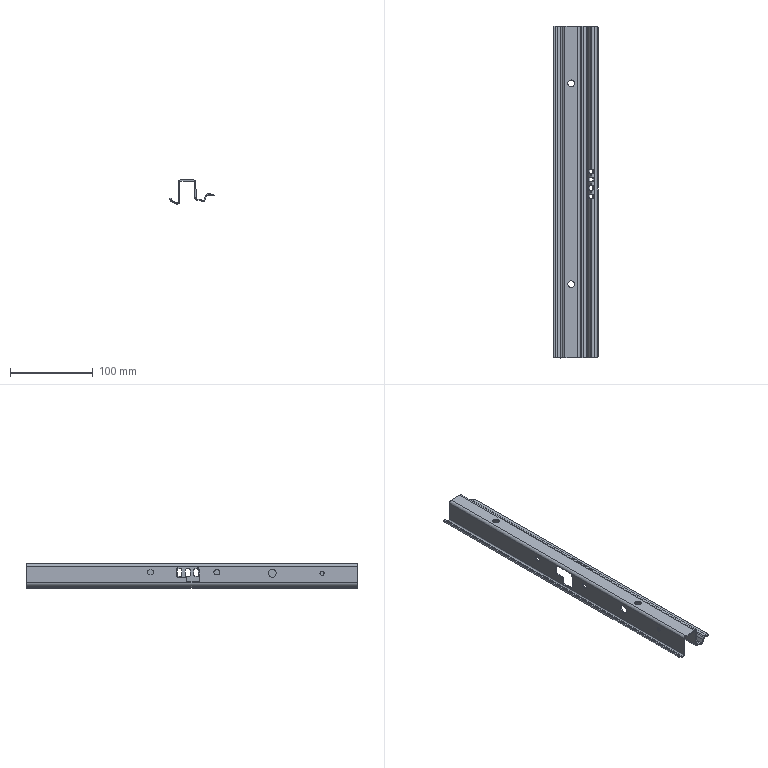Part | 1 solid | 327 faces | box 53.142 x 400 x 29.342 mm | volume 64872 mm3 | plane 129 | cylinder 88 | spline 74 | torus 24 | cone 12 | commonest cylinder face diameters 2 x17 1.36 x8 1.6 x8 4 x6 7.6 x5 10.7 x5